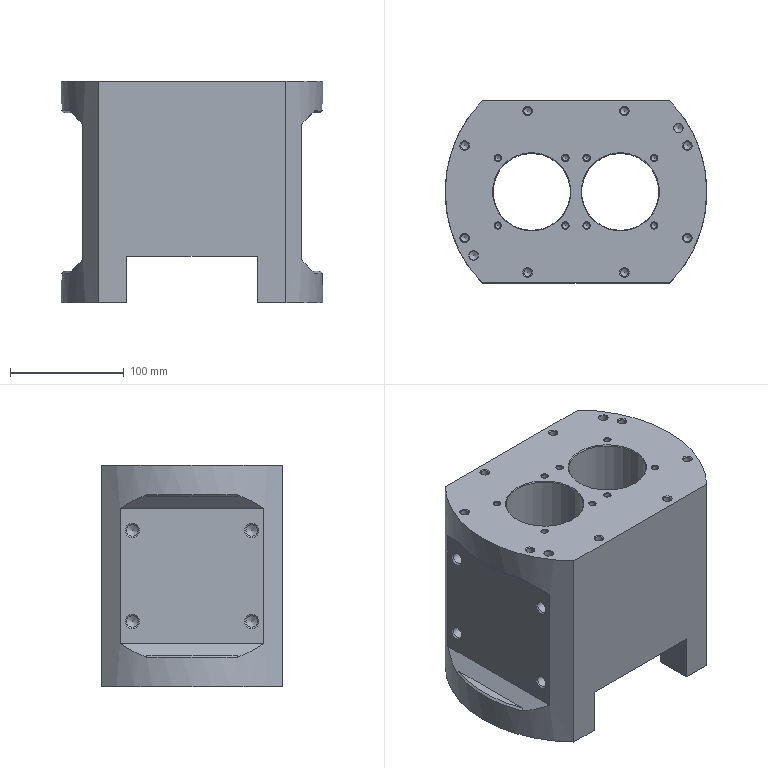NC program | NX | posted with a generic post | part box 230 x 160 x 195 mm
Whole program:
N10 G17 G21 G94 G90
(FLOOR_WALL , TOOL : D50)
N12 T02 M6
N14 G54
N16 G17 G0 G90 X-46.956 Y107.497 B0. C0. S1200 M3
N18 G43 Z30. H2
N20 Z2.651
N22 G94 G1 Z-0.349 F1000.
N24 X-43.956
N26 X43.956 F2000.
N28 Y68.498
N30 X-43.956
N32 Y29.498
N34 X43.956
N36 Y-9.501
N38 X-43.956
N40 Y-48.501
N42 X43.956
N44 Y-87.5
N46 X-43.956
N48 X-46.956
N50 Z2.651
N52 G0 Z30.
N54 X-50.654 Y107.497
N56 Z2.302
N58 G1 Z-0.698 F1000.
N60 X-47.654
N62 X47.654 F2000.
N64 Y68.498
N66 X-47.654
N68 Y29.498
N70 X47.654
N72 Y-9.501
N74 X-47.654
N76 Y-48.501
N78 X47.654
N80 Y-87.5
N82 X-47.654
N84 X-50.654
N86 Z2.302
N88 G0 Z30.
N90 X-53.485 Y107.497
N92 Z1.953
N94 G1 Z-1.047 F1000.
N96 X-50.485
N98 X50.485 F2000.
N100 Y68.498
N102 X-50.485
N104 Y29.498
N106 X50.485
N108 Y-9.501
N110 X-50.485
N112 Y-48.501
N114 X50.485
N116 Y-87.5
N118 X-50.485
N120 X-53.485
N122 Z1.953
N124 G0 Z30.
N126 X-55.866 Y107.497
N128 Z1.604
N130 G1 Z-1.396 F1000.
N132 X-52.866
N134 X52.866 F2000.
N136 Y68.498
N138 X-52.866
N140 Y29.498
N142 X52.866
N144 Y-9.501
N146 X-52.866
N148 Y-48.501
N150 X52.866
N152 Y-87.5
N154 X-52.866
N156 X-55.866
N158 Z1.604
N160 G0 Z30.
N162 X-57.959 Y107.497
N164 Z1.255
N166 G1 Z-1.745 F1000.
N168 X-54.959
N170 X54.959 F2000.
N172 Y68.498
N174 X-54.959
N176 Y29.498
N178 X54.959
N180 Y-9.501
N182 X-54.959
N184 Y-48.501
N186 X54.959
N188 Y-87.5
N190 X-54.959
N192 X-57.959
N194 Z1.255
N196 G0 Z30.
N198 X-59.847 Y107.497
N200 Z0.906
N202 G1 Z-2.094 F1000.
N204 X-56.847
N206 X56.847 F2000.
N208 Y68.498
N210 X-56.847
N212 Y29.498
N214 X56.847
N216 Y-9.501
N218 X-56.847
N220 Y-48.501
N222 X56.847
N224 Y-87.5
N226 X-56.847
N228 X-59.847
N230 Z0.906
N232 G0 Z30.
N234 X-61.579 Y107.497
N236 Z0.557
N238 G1 Z-2.443 F1000.
N240 X-58.579
N242 X58.579 F2000.
N244 Y68.498
N246 X-58.579
N248 Y29.498
N250 X58.579
N252 Y-9.501
N254 X-58.579
N256 Y-48.501
N258 X58.579
N260 Y-87.5
N262 X-58.579
N264 X-61.579
N266 Z0.557
N268 G0 Z30.
N270 X-63.188 Y107.497
N272 Z0.208
N274 G1 Z-2.792 F1000.
N276 X-60.188
N278 X60.188 F2000.
N280 Y68.498
N282 X-60.188
N284 Y29.498
N286 X60.188
N288 Y-9.501
N290 X-60.188
N292 Y-48.501
N294 X60.188
N296 Y-87.5
N298 X-60.188
N300 X-63.188
N302 Z0.208
N304 G0 Z30.
N306 X-64.695 Y107.497
N308 Z-0.141
N310 G1 Z-3.141 F1000.
N312 X-61.695
N314 X61.695 F2000.
N316 Y68.498
N318 X-61.695
N320 Y29.498
N322 X61.695
N324 Y-9.501
N326 X-61.695
N328 Y-48.501
N330 X61.695
N332 Y-87.5
N334 X-61.695
N336 X-64.695
N338 Z-0.141
N340 G0 Z30.
N342 X-66.117 Y107.497
N344 Z-0.49
N346 G1 Z-3.49 F1000.
N348 X-63.117
N350 X63.117 F2000.
N352 Y68.498
N354 X-63.117
N356 Y29.498
N358 X63.117
N360 Y-9.501
N362 X-63.117
N364 Y-48.501
N366 X63.117
N368 Y-87.5
N370 X-63.117
N372 X-66.117
N374 Z-0.49
N376 G0 Z30.
N378 X-67.467 Y107.497
N380 Z-0.839
N382 G1 Z-3.839 F1000.
N384 X-64.467
N386 X64.467 F2000.
N388 Y68.498
N390 X-64.467
N392 Y29.498
N394 X64.467
N396 Y-9.501
N398 X-64.467
N400 Y-48.501
N402 X64.467
N404 Y-87.5
N406 X-64.467
N408 X-67.467
N410 Z-0.839
N412 G0 Z30.
N414 X-68.753 Y107.497
N416 Z-1.188
N418 G1 Z-4.188 F1000.
N420 X-65.753
N422 X65.753 F2000.
N424 Y68.498
N426 X-65.753
N428 Y29.498
N430 X65.753
N432 Y-9.501
N434 X-65.753
N436 Y-48.501
N438 X65.753
N440 Y-87.5
N442 X-65.753
N444 X-68.753
N446 Z-1.188
N448 G0 Z30.
N450 X-69.984 Y107.497
N452 Z-1.537
N454 G1 Z-4.537 F1000.
N456 X-66.984
N458 X66.984 F2000.
N460 Y68.498
N462 X-66.984
N464 Y29.498
N466 X66.984
N468 Y-9.501
N470 X-66.984
N472 Y-48.501
N474 X66.984
N476 Y-87.5
N478 X-66.984
N480 X-69.984
N482 Z-1.537
N484 G0 Z30.
N486 X-71.166 Y107.497
N488 Z-1.886
N490 G1 Z-4.886 F1000.
N492 X-68.166
N494 X68.166 F2000.
N496 Y68.498
N498 X-68.166
N500 Y29.498
N502 X68.166
N504 Y-9.501
N506 X-68.166
N508 Y-48.501
N510 X68.166
N512 Y-87.5
N514 X-68.166
N516 X-71.166
N518 Z-1.886
N520 G0 Z30.
N522 X-72.303 Y107.497
N524 Z-2.235
N526 G1 Z-5.235 F1000.
N528 X-69.303
N530 X69.303 F2000.
N532 Y68.498
N534 X-69.303
N536 Y29.498
N538 X69.303
N540 Y-9.501
N542 X-69.303
N544 Y-48.501
N546 X69.303
N548 Y-87.5
N550 X-69.303
N552 X-72.303
N554 Z-2.235
N556 G0 Z30.
N558 X-73.4 Y107.497
N560 Z-2.584
N562 G1 Z-5.584 F1000.
N564 X-70.4
N566 X70.4 F2000.
N568 Y68.498
N570 X-70.4
N572 Y29.498
N574 X70.4
N576 Y-9.501
N578 X-70.4
N580 Y-48.501
N582 X70.4
N584 Y-87.5
N586 X-70.4
N588 X-73.4
N590 Z-2.584
N592 G0 Z30.
N594 X-74.462 Y107.497
N596 Z-2.933
N598 G1 Z-5.933 F1000.
N600 X-71.462
N602 X71.462 F2000.
N604 Y68.498
N606 X-71.462
N608 Y29.498
N610 X71.462
N612 Y-9.501
N614 X-71.462
N616 Y-48.501
N618 X71.462
N620 Y-87.5
N622 X-71.462
N624 X-74.462
N626 Z-2.933
N628 G0 Z30.
N630 X-75.489 Y107.497
N632 Z-3.282
N634 G1 Z-6.282 F1000.
N636 X-72.489
N638 X72.489 F2000.
N640 Y68.498
N642 X-72.489
N644 Y29.498
N646 X72.489
N648 Y-9.501
N650 X-72.489
N652 Y-48.501
N654 X72.489
N656 Y-87.5
N658 X-72.489
N660 X-75.489
N662 Z-3.282
N664 G0 Z30.
N666 X-76.487 Y107.497
N668 Z-3.631
N670 G1 Z-6.631 F1000.
N672 X-73.487
N674 X73.487 F2000.
N676 Y68.498
N678 X-73.487
N680 Y29.498
N682 X73.487
N684 Y-9.501
N686 X-73.487
N688 Y-48.501
N690 X73.487
N692 Y-87.5
N694 X-73.487
N696 X-76.487
N698 Z-3.631
N700 G0 Z30.
N702 X-77.455 Y107.497
N704 Z-3.98
N706 G1 Z-6.98 F1000.
N708 X-74.455
N710 X74.455 F2000.
N712 Y68.498
N714 X-74.455
N716 Y29.498
N718 X74.455
N720 Y-9.501
N722 X-74.455
N724 Y-48.501
N726 X74.455
N728 Y-87.5
N730 X-74.455
N732 X-77.455
N734 Z-3.98
N736 G0 Z30.
N738 X-78.398 Y107.497
N740 Z-4.329
N742 G1 Z-7.329 F1000.
N744 X-75.398
N746 X75.398 F2000.
N748 Y68.498
N750 X-75.398
N752 Y29.498
N754 X75.398
N756 Y-9.501
N758 X-75.398
N760 Y-48.501
N762 X75.398
N764 Y-87.5
N766 X-75.398
N768 X-78.398
N770 Z-4.329
N772 G0 Z30.
N774 X-79.316 Y107.497
N776 Z-4.678
N778 G1 Z-7.678 F1000.
N780 X-76.316
N782 X76.316 F2000.
N784 Y68.498
N786 X-76.316
N788 Y29.498
N790 X76.316
N792 Y-9.501
N794 X-76.316
N796 Y-48.501
N798 X76.316
N800 Y-87.5
N802 X-76.316
N804 X-79.316
N806 Z-4.678
N808 G0 Z30.
N810 X-80.212 Y107.497
N812 Z-5.027
N814 G1 Z-8.027 F1000.
N816 X-77.212
N818 X77.212 F2000.
N820 Y68.498
N822 X-77.212
N824 Y29.498
N826 X77.212
N828 Y-9.501
N830 X-77.212
N832 Y-48.501
N834 X77.212
N836 Y-87.5
N838 X-77.212
N840 X-80.212
N842 Z-5.027
N844 G0 Z30.
N846 X-81.086 Y107.497
N848 Z-5.376
N850 G1 Z-8.376 F1000.
N852 X-78.086
N854 X78.086 F2000.
N856 Y68.498
N858 X-78.086
N860 Y29.498
N862 X78.086
N864 Y-9.501
N866 X-78.086
N868 Y-48.501
N870 X78.086
N872 Y-87.5
N874 X-78.086
N876 X-81.086
N878 Z-5.376
N880 G0 Z30.
N882 X-81.939 Y107.497
N884 Z-5.725
N886 G1 Z-8.725 F1000.
N888 X-78.939
N890 X78.939 F2000.
N892 Y68.498
N894 X-78.939
N896 Y29.498
N898 X78.939
N900 Y-9.501
N902 X-78.939
N904 Y-48.501
N906 X78.939
N908 Y-87.5
N910 X-78.939
N912 X-81.939
N914 Z-5.725
N916 G0 Z30.
N918 X-82.774 Y107.497
N920 Z-6.074
N922 G1 Z-9.074 F1000.
N924 X-79.774
N926 X79.774 F2000.
N928 Y68.498
N930 X-79.774
N932 Y29.498
N934 X79.774
N936 Y-9.501
N938 X-79.774
N940 Y-48.501
N942 X79.774
N944 Y-87.5
N946 X-79.774
N948 X-82.774
N950 Z-6.074
N952 G0 Z30.
N954 X-83.591 Y107.497
N956 Z-6.423
N958 G1 Z-9.423 F1000.
N960 X-80.591
N962 X80.591 F2000.
N964 Y68.498
N966 X-80.591
N968 Y29.498
N970 X80.591
N972 Y-9.501
N974 X-80.591
N976 Y-48.501
N978 X80.591
N980 Y-87.5
N982 X-80.591
N984 X-83.591
N986 Z-6.423
N988 G0 Z30.
N990 X-84.391 Y107.497
N992 Z-6.772
N994 G1 Z-9.772 F1000.
N996 X-81.391
N998 X81.391 F2000.
N1000 Y68.498
N1002 X-81.391
N1004 Y29.498
N1006 X81.391
N1008 Y-9.501
N1010 X-81.391
N1012 Y-48.501
N1014 X81.391
N1016 Y-87.5
N1018 X-81.391
N1020 X-84.391
N1022 Z-6.772
N1024 G0 Z30.
N1026 X-85.175 Y107.497
N1028 Z-7.121
N1030 G1 Z-10.121 F1000.
N1032 X-82.175
N1034 X82.175 F2000.
N1036 Y68.498
N1038 X-82.175
N1040 Y29.498
N1042 X82.175
N1044 Y-9.501
N1046 X-82.175
N1048 Y-48.501
N1050 X82.175
N1052 Y-87.5
N1054 X-82.175
N1056 X-85.175
N1058 Z-7.121
N1060 G0 Z30.
N1062 X-85.943 Y107.497
N1064 Z-7.47
N1066 G1 Z-10.47 F1000.
N1068 X-82.943
N1070 X82.943 F2000.
N1072 Y68.498
N1074 X-82.943
N1076 Y29.498
N1078 X82.943
N1080 Y-9.501
N1082 X-82.943
N1084 Y-48.501
N1086 X82.943
N1088 Y-87.5
N1090 X-82.943
N1092 X-85.943
N1094 Z-7.47
N1096 G0 Z30.
N1098 X-86.697 Y107.497
N1100 Z-7.819
N1102 G1 Z-10.819 F1000.
N1104 X-83.697
N1106 X83.697 F2000.
N1108 Y68.498
N1110 X-83.697
N1112 Y29.498
N1114 X83.697
N1116 Y-9.501
N1118 X-83.697
N1120 Y-48.501
N1122 X83.697
N1124 Y-87.5
N1126 X-83.697
N1128 X-86.697
N1130 Z-7.819
N1132 G0 Z30.
N1134 X-87.436 Y107.497
N1136 Z-8.168
N1138 G1 Z-11.168 F1000.
N1140 X-84.436
N1142 X84.436 F2000.
N1144 Y68.498
N1146 X-84.436
N1148 Y29.498
N1150 X84.436
N1152 Y-9.501
N1154 X-84.436
N1156 Y-48.501
N1158 X84.436
N1160 Y-87.5
N1162 X-84.436
N1164 X-87.436
N1166 Z-8.168
N1168 G0 Z30.
N1170 X-88.163 Y107.497
N1172 Z-8.517
N1174 G1 Z-11.517 F1000.
N1176 X-85.163
N1178 X85.163 F2000.
N1180 Y68.498
N1182 X-85.163
N1184 Y29.498
N1186 X85.163
N1188 Y-9.501
N1190 X-85.163
N1192 Y-48.501
N1194 X85.163
N1196 Y-87.5
N1198 X-85.163
N1200 X-88.163
N1202 Z-8.517
N1204 G0 Z30.
N1206 X-88.877 Y107.497
N1208 Z-8.866
N1210 G1 Z-11.866 F1000.
N1212 X-85.877
N1214 X85.877 F2000.
N1216 Y68.498
N1218 X-85.877
N1220 Y29.498
N1222 X85.877
N1224 Y-9.501
N1226 X-85.877
N1228 Y-48.501
N1230 X85.877
N1232 Y-87.5
N1234 X-85.877
N1236 X-88.877
N1238 Z-8.866
N1240 G0 Z30.
N1242 X-89.578 Y107.497
N1244 Z-9.215
N1246 G1 Z-12.215 F1000.
N1248 X-86.578
N1250 X86.578 F2000.
N1252 Y68.498
N1254 X-86.578
N1256 Y29.498
N1258 X86.578
N1260 Y-9.501
N1262 X-86.578
N1264 Y-48.501
N1266 X86.578
N1268 Y-87.5
N1270 X-86.578
N1272 X-89.578
N1274 Z-9.215
N1276 G0 Z30.
N1278 X-90.268 Y107.497
N1280 Z-9.564
N1282 G1 Z-12.564 F1000.
N1284 X-87.268
N1286 X87.268 F2000.
N1288 Y68.498
N1290 X-87.268
N1292 Y29.498
N1294 X87.268
N1296 Y-9.501
N1298 X-87.268
N1300 Y-48.501
N1302 X87.268
N1304 Y-87.5
N1306 X-87.268
N1308 X-90.268
N1310 Z-9.564
N1312 G0 Z30.
N1314 X-90.946 Y107.497
N1316 Z-9.913
N1318 G1 Z-12.913 F1000.
N1320 X-87.946
N1322 X87.946 F2000.
N1324 Y68.498
N1326 X-87.946
N1328 Y29.498
N1330 X87.946
N1332 Y-9.501
N1334 X-87.946
N1336 Y-48.501
N1338 X87.946
N1340 Y-87.5
N1342 X-87.946
N1344 X-90.946
N1346 Z-9.913
N1348 G0 Z30.
N1350 X-91.614 Y107.497
N1352 Z-10.262
N1354 G1 Z-13.262 F1000.
N1356 X-88.614
N1358 X88.614 F2000.
N1360 Y68.498
N1362 X-88.614
N1364 Y29.498
N1366 X88.614
N1368 Y-9.501
N1370 X-88.614
N1372 Y-48.501
N1374 X88.614
N1376 Y-87.5
N1378 X-88.614
N1380 X-91.614
N1382 Z-10.262
N1384 G0 Z30.
N1386 X-92.271 Y107.497
N1388 Z-10.611
N1390 G1 Z-13.611 F1000.
N1392 X-89.271
N1394 X89.271 F2000.
N1396 Y68.498
N1398 X-89.271
N1400 Y29.498
N1402 X89.271
N1404 Y-9.501
N1406 X-89.271
N1408 Y-48.501
N1410 X89.271
N1412 Y-87.5
N1414 X-89.271
N1416 X-92.271
N1418 Z-10.611
N1420 G0 Z30.
N1422 X-92.918 Y107.497
N1424 Z-10.96
N1426 G1 Z-13.96 F1000.
N1428 X-89.918
N1430 X89.918 F2000.
N1432 Y68.498
N1434 X-89.918
N1436 Y29.498
N1438 X89.918
N1440 Y-9.501
N1442 X-89.918
N1444 Y-48.501
N1446 X89.918
N1448 Y-87.5
N1450 X-89.918
N1452 X-92.918
N1454 Z-10.96
N1456 G0 Z30.
N1458 X-93.555 Y107.497
N1460 Z-11.309
N1462 G1 Z-14.309 F1000.
N1464 X-90.555
N1466 X90.555 F2000.
N1468 Y68.498
N1470 X-90.555
N1472 Y29.498
N1474 X90.555
N1476 Y-9.501
N1478 X-90.555
N1480 Y-48.501
N1482 X90.555
N1484 Y-87.5
N1486 X-90.555
N1488 X-93.555
N1490 Z-11.309
N1492 G0 Z30.
N1494 X-94.183 Y107.497
N1496 Z-11.658
N1498 G1 Z-14.658 F1000.
N1500 X-91.183
N1502 X91.183 F2000.
N1504 Y68.498
N1506 X-91.183
N1508 Y29.498
N1510 X91.183
N1512 Y-9.501
N1514 X-91.183
N1516 Y-48.501
N1518 X91.183
N1520 Y-87.5
N1522 X-91.183
N1524 X-94.183
N1526 Z-11.658
N1528 G0 Z30.
N1530 X-94.802 Y107.497
N1532 Z-12.007
N1534 G1 Z-15.007 F1000.
N1536 X-91.802
N1538 X91.802 F2000.
N1540 Y68.498
N1542 X-91.802
N1544 Y29.498
N1546 X91.802
N1548 Y-9.501
N1550 X-91.802
N1552 Y-48.501
N1554 X91.802
N1556 Y-87.5
N1558 X-91.802
N1560 X-94.802
N1562 Z-12.007
N1564 G0 Z30.
N1566 X-95.412 Y107.497
N1568 Z-12.356
N1570 G1 Z-15.356 F1000.
N1572 X-92.412
N1574 X92.412 F2000.
N1576 Y68.498
N1578 X-92.412
N1580 Y29.498
N1582 X92.412
N1584 Y-9.501
N1586 X-92.412
N1588 Y-48.501
N1590 X92.412
N1592 Y-87.5
N1594 X-92.412
N1596 X-95.412
N1598 Z-12.356
N1600 G0 Z30.
N1602 X-96.013 Y107.497
N1604 Z-12.705
N1606 G1 Z-15.705 F1000.
N1608 X-93.013
N1610 X93.013 F2000.
N1612 Y68.498
N1614 X-93.013
N1616 Y29.498
N1618 X93.013
N1620 Y-9.501
N1622 X-93.013
N1624 Y-48.501
N1626 X93.013
N1628 Y-87.5
N1630 X-93.013
N1632 X-96.013
N1634 Z-12.705
N1636 G0 Z30.
N1638 X-96.606 Y107.497
N1640 Z-13.054
N1642 G1 Z-16.054 F1000.
N1644 X-93.606
N1646 X93.606 F2000.
N1648 Y68.498
N1650 X-93.606
N1652 Y29.498
N1654 X93.606
N1656 Y-9.501
N1658 X-93.606
N1660 Y-48.501
N1662 X93.606
N1664 Y-87.5
N1666 X-93.606
N1668 X-96.606
N1670 Z-13.054
N1672 G0 Z30.
N1674 X-97.192 Y107.497
N1676 Z-13.403
N1678 G1 Z-16.403 F1000.
N1680 X-94.192
N1682 X94.192 F2000.
N1684 Y68.498
N1686 X-94.192
N1688 Y29.498
N1690 X94.192
N1692 Y-9.501
N1694 X-94.192
N1696 Y-48.501
N1698 X94.192
N1700 Y-87.5
N1702 X-94.192
N1704 X-97.192
N1706 Z-13.403
N1708 G0 Z30.
N1710 X-97.769 Y107.497
N1712 Z-13.752
N1714 G1 Z-16.752 F1000.
N1716 X-94.769
N1718 X94.769 F2000.
N1720 Y68.498
N1722 X-94.769
N1724 Y29.498
N1726 X94.769
N1728 Y-9.501
N1730 X-94.769
N1732 Y-48.501
N1734 X94.769
N1736 Y-87.5
N1738 X-94.769
N1740 X-97.769
N1742 Z-13.752
N1744 G0 Z30.
N1746 X-98.339 Y107.497
N1748 Z-14.101
N1750 G1 Z-17.101 F1000.
N1752 X-95.339
N1754 X95.339 F2000.
N1756 Y68.498
N1758 X-95.339
N1760 Y29.498
N1762 X95.339
N1764 Y-9.501
N1766 X-95.339
N1768 Y-48.501
N1770 X95.339
N1772 Y-87.5
N1774 X-95.339
N1776 X-98.339
N1778 Z-14.101
N1780 G0 Z30.
N1782 X-98.902 Y107.497
N1784 Z-14.45
N1786 G1 Z-17.45 F1000.
N1788 X-95.902
N1790 X95.902 F2000.
N1792 Y68.498
N1794 X-95.902
N1796 Y29.498
N1798 X95.902
N1800 Y-9.501
N1802 X-95.902
N1804 Y-48.501
N1806 X95.902
N1808 Y-87.5
N1810 X-95.902
N1812 X-98.902
N1814 Z-14.45
N1816 G0 Z30.
N1818 X-99.457 Y107.497
N1820 Z-14.799
N1822 G1 Z-17.799 F1000.
N1824 X-96.457
N1826 X96.457 F2000.
N1828 Y68.498
N1830 X-96.457
N1832 Y29.498
N1834 X96.457
N1836 Y-9.501
N1838 X-96.457
N1840 Y-48.501
N1842 X96.457
N1844 Y-87.5
N1846 X-96.457
N1848 X-99.457
N1850 Z-14.799
N1852 G0 Z30.
N1854 X-100.006 Y107.497
N1856 Z-15.148
N1858 G1 Z-18.148 F1000.
N1860 X-97.006
N1862 X97.006 F2000.
N1864 Y68.498
N1866 X-97.006
N1868 Y29.498
N1870 X97.006
N1872 Y-9.501
N1874 X-97.006
N1876 Y-48.501
N1878 X97.006
N1880 Y-87.5
N1882 X-97.006
N1884 X-100.006
N1886 Z-15.148
N1888 G0 Z30.
N1890 X-100.548 Y107.497
N1892 Z-15.497
N1894 G1 Z-18.497 F1000.
N1896 X-97.548
N1898 X97.548 F2000.
N1900 Y68.498
N1902 X-97.548
N1904 Y29.498
N1906 X97.548
N1908 Y-9.501
N1910 X-97.548
N1912 Y-48.501
N1914 X97.548
N1916 Y-87.5
N1918 X-97.548
N1920 X-100.548
N1922 Z-15.497
N1924 G0 Z30.
N1926 X-101.083 Y107.497
N1928 Z-15.846
N1930 G1 Z-18.846 F1000.
N1932 X-98.083
N1934 X98.083 F2000.
N1936 Y68.498
N1938 X-98.083
N1940 Y29.498
N1942 X98.083
N1944 Y-9.501
N1946 X-98.083
N1948 Y-48.501
N1950 X98.083
N1952 Y-87.5
N1954 X-98.083
N1956 X-101.083
N1958 Z-15.846
N1960 G0 Z30.
N1962 X-101.612 Y107.497
N1964 Z-16.195
N1966 G1 Z-19.195 F1000.
N1968 X-98.612
N1970 X98.612 F2000.
N1972 Y68.498
N1974 X-98.612
N1976 Y29.498
N1978 X98.612
N1980 Y-9.501
N1982 X-98.612
N1984 Y-48.501
N1986 X98.612
N1988 Y-87.5
N1990 X-98.612
N1992 X-101.612
N1994 Z-16.195
N1996 G0 Z30.
N1998 X-102.134 Y107.497
N2000 Z-16.544
N2002 G1 Z-19.544 F1000.
N2004 X-99.134
N2006 X99.134 F2000.
N2008 Y68.498
N2010 X-99.134
N2012 Y29.498
N2014 X99.134
N2016 Y-9.501
N2018 X-99.134
N2020 Y-48.501
N2022 X99.134
N2024 Y-87.5
N2026 X-99.134
N2028 X-102.134
N2030 Z-16.544
N2032 G0 Z30.
N2034 X-102.65 Y107.497
N2036 Z-16.893
N2038 G1 Z-19.893 F1000.
N2040 X-99.65
N2042 X99.65 F2000.
N2044 Y68.498
N2046 X-99.65
N2048 Y29.498
N2050 X99.65
N2052 Y-9.501
N2054 X-99.65
N2056 Y-48.501
N2058 X99.65
N2060 Y-87.5
N2062 X-99.65
N2064 X-102.65
N2066 Z-16.893
N2068 G0 Z30.
N2070 X-103.161 Y107.497
N2072 Z-17.242
N2074 G1 Z-20.242 F1000.
N2076 X-100.161
N2078 X100.161 F2000.
N2080 Y68.498
N2082 X-100.161
N2084 Y29.498
N2086 X100.161
N2088 Y-9.501
N2090 X-100.161
N2092 Y-48.501
N2094 X100.161
N2096 Y-87.5
N2098 X-100.161
N2100 X-103.161
N2102 Z-17.242
N2104 G0 Z30.
N2106 X-103.666 Y107.497
N2108 Z-17.591
N2110 G1 Z-20.591 F1000.
N2112 X-100.666
N2114 X100.666 F2000.
N2116 Y68.498
N2118 X-100.666
N2120 Y29.498
N2122 X100.666
N2124 Y-9.501
N2126 X-100.666
N2128 Y-48.501
N2130 X100.666
N2132 Y-87.5
N2134 X-100.666
N2136 X-103.666
N2138 Z-17.591
N2140 G0 Z30.
N2142 X-104.164 Y107.497
N2144 Z-17.94
N2146 G1 Z-20.94 F1000.
N2148 X-101.164
N2150 X101.164 F2000.
N2152 Y68.498
N2154 X-101.164
N2156 Y29.498
N2158 X101.164
N2160 Y-9.501
N2162 X-101.164
N2164 Y-48.501
N2166 X101.164
N2168 Y-87.5
N2170 X-101.164
N2172 X-104.164
N2174 Z-17.94
N2176 G0 Z30.
N2178 X-104.658 Y107.497
N2180 Z-18.289
N2182 G1 Z-21.289 F1000.
N2184 X-101.658
N2186 X101.658 F2000.
N2188 Y68.498
N2190 X-101.658
N2192 Y29.498
N2194 X101.658
N2196 Y-9.501
N2198 X-101.658
N2200 Y-48.501
N2202 X101.658
N2204 Y-87.5
N2206 X-101.658
N2208 X-104.658
N2210 Z-18.289
N2212 G0 Z30.
N2214 X-105.146 Y107.497
N2216 Z-18.638
N2218 G1 Z-21.638 F1000.
N2220 X-102.146
N2222 X102.146 F2000.
N2224 Y68.498
N2226 X-102.146
N2228 Y29.498
N2230 X102.146
N2232 Y-9.501
N2234 X-102.146
N2236 Y-48.501
N2238 X102.146
N2240 Y-87.5
N2242 X-102.146
N2244 X-105.146
N2246 Z-18.638
N2248 G0 Z30.
N2250 X-105.628 Y107.497
N2252 Z-18.987
N2254 G1 Z-21.987 F1000.
N2256 X-102.628
N2258 X102.628 F2000.
N2260 Y68.498
N2262 X-102.628
N2264 Y29.498
N2266 X102.628
N2268 Y-9.501
N2270 X-102.628
N2272 Y-48.501
N2274 X102.628
N2276 Y-87.5
N2278 X-102.628
N2280 X-105.628
N2282 Z-18.987
N2284 G0 Z30.
N2286 X-106.106 Y107.497
N2288 Z-19.336
N2290 G1 Z-22.336 F1000.
N2292 X-103.106
N2294 X103.106 F2000.
N2296 Y68.498
N2298 X-103.106
N2300 Y29.498
N2302 X103.106
N2304 Y-9.501
N2306 X-103.106
N2308 Y-48.501
N2310 X103.106
N2312 Y-87.5
N2314 X-103.106
N2316 X-106.106
N2318 Z-19.336
N2320 G0 Z30.
N2322 X-106.578 Y107.497
N2324 Z-19.685
N2326 G1 Z-22.685 F1000.
N2328 X-103.578
N2330 X103.578 F2000.
N2332 Y68.498
N2334 X-103.578
N2336 Y29.498
N2338 X103.578
N2340 Y-9.501
N2342 X-103.578
N2344 Y-48.501
N2346 X103.578
N2348 Y-87.5
N2350 X-103.578
N2352 X-106.578
N2354 Z-19.685
N2356 G0 Z30.
N2358 X-107.045 Y107.497
N2360 Z-20.034
N2362 G1 Z-23.034 F1000.
N2364 X-104.045
N2366 X104.045 F2000.
N2368 Y68.498
N2370 X-104.045
N2372 Y29.498
N2374 X104.045
N2376 Y-9.501
N2378 X-104.045
N2380 Y-48.501
N2382 X104.045
N2384 Y-87.5
N2386 X-104.045
N2388 X-107.045
N2390 Z-20.034
N2392 G0 Z30.
N2394 X-107.508 Y107.497
N2396 Z-20.383
N2398 G1 Z-23.383 F1000.
N2400 X-104.508
N2402 X104.508 F2000.
N2404 Y68.498
N2406 X-104.508
N2408 Y29.498
N2410 X104.508
N2412 Y-9.501
N2414 X-104.508
N2416 Y-48.501
N2418 X104.508
N2420 Y-87.5
N2422 X-104.508
N2424 X-107.508
N2426 Z-20.383
N2428 G0 Z30.
N2430 X-107.965 Y107.497
N2432 Z-20.732
N2434 G1 Z-23.732 F1000.
N2436 X-104.965
N2438 X104.965 F2000.
N2440 Y68.498
N2442 X-104.965
N2444 Y29.498
N2446 X104.965
N2448 Y-9.501
N2450 X-104.965
N2452 Y-48.501
N2454 X104.965
N2456 Y-87.5
N2458 X-104.965
N2460 X-107.965
N2462 Z-20.732
N2464 G0 Z30.
N2466 X-108.418 Y107.497
N2468 Z-21.081
N2470 G1 Z-24.081 F1000.
N2472 X-105.418
N2474 X105.418 F2000.
N2476 Y68.498
N2478 X-105.418
N2480 Y29.498
N2482 X105.418
N2484 Y-9.501
N2486 X-105.418
N2488 Y-48.501
N2490 X105.418
N2492 Y-87.5
N2494 X-105.418
N2496 X-108.418
N2498 Z-21.081
N2500 G0 Z30.
N2502 X-108.867 Y107.497
N2504 Z-21.43
N2506 G1 Z-24.43 F1000.
N2508 X-105.867
N2510 X105.867 F2000.
N2512 Y68.498
N2514 X-105.867
N2516 Y29.498
N2518 X105.867
N2520 Y-9.501
N2522 X-105.867
N2524 Y-48.501
N2526 X105.867
N2528 Y-87.5
N2530 X-105.867
N2532 X-108.867
N2534 Z-21.43
N2536 G0 Z30.
N2538 X-109.31 Y107.497
N2540 Z-21.779
N2542 G1 Z-24.779 F1000.
N2544 X-106.31
N2546 X106.31 F2000.
N2548 Y68.498
N2550 X-106.31
N2552 Y29.498
N2554 X106.31
N2556 Y-9.501
N2558 X-106.31
N2560 Y-48.501
N2562 X106.31
N2564 Y-87.5
N2566 X-106.31
N2568 X-109.31
N2570 Z-21.779
N2572 G0 Z30.
N2574 X-109.75 Y107.497
N2576 Z-22.128
N2578 G1 Z-25.128 F1000.
N2580 X-106.75
N2582 X106.75 F2000.
N2584 Y68.498
N2586 X-106.75
N2588 Y29.498
N2590 X106.75
N2592 Y-9.501
N2594 X-106.75
N2596 Y-48.501
N2598 X106.75
N2600 Y-87.5
N2602 X-106.75
N2604 X-109.75
N2606 Z-22.128
N2608 G0 Z30.
N2610 X-110.185 Y107.497
N2612 Z-22.477
N2614 G1 Z-25.477 F1000.
N2616 X-107.185
N2618 X107.185 F2000.
N2620 Y68.498
N2622 X-107.185
N2624 Y29.498
N2626 X107.185
N2628 Y-9.501
N2630 X-107.185
N2632 Y-48.501
N2634 X107.185
N2636 Y-87.5
N2638 X-107.185
N2640 X-110.185
N2642 Z-22.477
N2644 G0 Z30.
N2646 X-110.616 Y107.497
N2648 Z-22.826
N2650 G1 Z-25.826 F1000.
N2652 X-107.616
N2654 X107.616 F2000.
N2656 Y68.498
N2658 X-107.616
N2660 Y29.498
N2662 X107.616
N2664 Y-9.501
N2666 X-107.616
N2668 Y-48.501
N2670 X107.616
N2672 Y-87.5
N2674 X-107.616
N2676 X-110.616
N2678 Z-22.826
N2680 G0 Z30.
N2682 X-111.042 Y107.497
N2684 Z-23.175
N2686 G1 Z-26.175 F1000.
N2688 X-108.042
N2690 X108.042 F2000.
N2692 Y68.498
N2694 X-108.042
N2696 Y29.498
N2698 X108.042
N2700 Y-9.501
N2702 X-108.042
N2704 Y-48.501
N2706 X108.042
N2708 Y-87.5
N2710 X-108.042
N2712 X-111.042
N2714 Z-23.175
N2716 G0 Z30.
N2718 X-111.464 Y107.497
N2720 Z-23.524
N2722 G1 Z-26.524 F1000.
N2724 X-108.464
N2726 X108.464 F2000.
N2728 Y68.498
N2730 X-108.464
N2732 Y29.498
N2734 X108.464
N2736 Y-9.501
N2738 X-108.464
N2740 Y-48.501
N2742 X108.464
N2744 Y-87.5
N2746 X-108.464
N2748 X-111.464
N2750 Z-23.524
N2752 G0 Z30.
N2754 X-111.883 Y107.497
N2756 Z-23.873
N2758 G1 Z-26.873 F1000.
N2760 X-108.883
N2762 X108.883 F2000.
N2764 Y68.498
N2766 X-108.883
N2768 Y29.498
N2770 X108.883
N2772 Y-9.501
N2774 X-108.883
N2776 Y-48.501
N2778 X108.883
N2780 Y-87.5
N2782 X-108.883
N2784 X-111.883
N2786 Z-23.873
N2788 G0 Z30.
N2790 X-112.297 Y107.497
N2792 Z-24.222
N2794 G1 Z-27.222 F1000.
N2796 X-109.297
N2798 X109.297 F2000.
N2800 Y68.498
N2802 X-109.297
N2804 Y29.498
N2806 X109.297
N2808 Y-9.501
N2810 X-109.297
N2812 Y-48.501
N2814 X109.297
N2816 Y-87.5
N2818 X-109.297
N2820 X-112.297
N2822 Z-24.222
N2824 G0 Z30.
N2826 X-112.707 Y107.497
N2828 Z-24.571
N2830 G1 Z-27.571 F1000.
N2832 X-109.707
N2834 X109.707 F2000.
N2836 Y68.498
N2838 X-109.707
N2840 Y29.498
N2842 X109.707
N2844 Y-9.501
N2846 X-109.707
N2848 Y-48.501
N2850 X109.707
N2852 Y-87.5
N2854 X-109.707
N2856 X-112.707
N2858 Z-24.571
N2860 G0 Z30.
N2862 X-113.114 Y107.497
N2864 Z-24.92
N2866 G1 Z-27.92 F1000.
N2868 X-110.114
N2870 X110.114 F2000.
N2872 Y68.498
N2874 X-110.114
N2876 Y29.498
N2878 X110.114
N2880 Y-9.501
N2882 X-110.114
N2884 Y-48.501
N2886 X110.114
N2888 Y-87.5
N2890 X-110.114
N2892 X-113.114
N2894 Z-24.92
N2896 G0 Z30.
N2898 X-113.517 Y107.497
N2900 Z-25.269
N2902 G1 Z-28.269 F1000.
N2904 X-110.517
N2906 X110.517 F2000.
N2908 Y68.498
N2910 X-110.517
N2912 Y29.498
N2914 X110.517
N2916 Y-9.501
N2918 X-110.517
N2920 Y-48.501
N2922 X110.517
N2924 Y-87.5
N2926 X-110.517
N2928 X-113.517
N2930 Z-25.269
N2932 G0 Z30.
N2934 X-113.915 Y107.497
N2936 Z-25.618
N2938 G1 Z-28.618 F1000.
N2940 X-110.915
N2942 X110.915 F2000.
N2944 Y68.498
N2946 X-110.915
N2948 Y29.498
N2950 X110.915
N2952 Y-9.501
N2954 X-110.915
N2956 Y-48.501
N2958 X110.915
N2960 Y-87.5
N2962 X-110.915
N2964 X-113.915
N2966 Z-25.618
N2968 G0 Z30.
N2970 X-114.311 Y107.497
N2972 Z-25.967
N2974 G1 Z-28.967 F1000.
N2976 X-111.311
N2978 X111.311 F2000.
N2980 Y68.498
N2982 X-111.311
N2984 Y29.498
N2986 X111.311
N2988 Y-9.501
N2990 X-111.311
N2992 Y-48.501
N2994 X111.311
N2996 Y-87.5
N2998 X-111.311
N3000 X-114.311
N3002 Z-25.967
N3004 G0 Z30.
N3006 X-114.702 Y107.497
N3008 Z-26.316
N3010 G1 Z-29.316 F1000.
N3012 X-111.702
N3014 X111.702 F2000.
N3016 Y68.498
N3018 X-111.702
N3020 Y29.498
N3022 X111.702
N3024 Y-9.501
N3026 X-111.702
N3028 Y-48.501
N3030 X111.702
N3032 Y-87.5
N3034 X-111.702
N3036 X-114.702
N3038 Z-26.316
N3040 G0 Z30.
N3042 X-115.091 Y107.497
N3044 Z-26.665
N3046 G1 Z-29.665 F1000.
N3048 X-112.091
N3050 X112.091 F2000.
N3052 Y68.498
N3054 X-112.091
N3056 Y29.498
N3058 X112.091
N3060 Y-9.501
N3062 X-112.091
N3064 Y-48.501
N3066 X112.091
N3068 Y-87.5
N3070 X-112.091
N3072 X-115.091
N3074 Z-26.665
N3076 G0 Z30.
N3078 X-115.475 Y107.497
N3080 Z-27.014
N3082 G1 Z-30.014 F1000.
N3084 X-112.475
N3086 X112.475 F2000.
N3088 Y68.498
N3090 X-112.475
N3092 Y29.498
N3094 X112.475
N3096 Y-9.501
N3098 X-112.475
N3100 Y-48.501
N3102 X112.475
N3104 Y-87.5
N3106 X-112.475
N3108 X-115.475
N3110 Z-27.014
N3112 G0 Z30.
N3114 X-115.856 Y107.497
N3116 Z-27.363
N3118 G1 Z-30.363 F1000.
N3120 X-112.856
N3122 X112.856 F2000.
N3124 Y68.498
N3126 X-112.856
N3128 Y29.498
N3130 X112.856
N3132 Y-9.501
N3134 X-112.856
N3136 Y-48.501
N3138 X112.856
N3140 Y-87.5
N3142 X-112.856
N3144 X-115.856
N3146 Z-27.363
N3148 G0 Z30.
N3150 X-116.234 Y107.497
N3152 Z-27.712
N3154 G1 Z-30.712 F1000.
N3156 X-113.234
N3158 X113.234 F2000.
N3160 Y68.498
N3162 X-113.234
N3164 Y29.498
N3166 X113.234
N3168 Y-9.501
N3170 X-113.234
N3172 Y-48.501
N3174 X113.234
N3176 Y-87.5
N3178 X-113.234
N3180 X-116.234
N3182 Z-27.712
N3184 G0 Z30.
N3186 X-116.608 Y107.497
N3188 Z-28.061
N3190 G1 Z-31.061 F1000.
N3192 X-113.608
N3194 X113.608 F2000.
N3196 Y68.498
N3198 X-113.608
N3200 Y29.498
N3202 X113.608
N3204 Y-9.501
N3206 X-113.608
N3208 Y-48.501
N3210 X113.608
N3212 Y-87.5
N3214 X-113.608
N3216 X-116.608
N3218 Z-28.061
N3220 G0 Z30.
N3222 X-116.979 Y107.497
N3224 Z-28.41
N3226 G1 Z-31.41 F1000.
N3228 X-113.979
N3230 X113.979 F2000.
N3232 Y68.498
N3234 X-113.979
N3236 Y29.498
N3238 X113.979
N3240 Y-9.501
N3242 X-113.979
N3244 Y-48.501
N3246 X113.979
N3248 Y-87.5
N3250 X-113.979
N3252 X-116.979
N3254 Z-28.41
N3256 G0 Z30.
N3258 X-117.347 Y107.497
N3260 Z-28.759
N3262 G1 Z-31.759 F1000.
N3264 X-114.347
N3266 X114.347 F2000.
N3268 Y68.498
N3270 X-114.347
N3272 Y29.498
N3274 X114.347
N3276 Y-9.501
N3278 X-114.347
N3280 Y-48.501
N3282 X114.347
N3284 Y-87.5
N3286 X-114.347
N3288 X-117.347
N3290 Z-28.759
N3292 G0 Z30.
N3294 X-117.711 Y107.497
N3296 Z-29.108
N3298 G1 Z-32.108 F1000.
N3300 X-114.711
N3302 X114.711 F2000.
N3304 Y68.498
N3306 X-114.711
N3308 Y29.498
N3310 X114.711
N3312 Y-9.501
N3314 X-114.711
N3316 Y-48.501
N3318 X114.711
N3320 Y-87.5
N3322 X-114.711
N3324 X-117.711
N3326 Z-29.108
N3328 G0 Z30.
N3330 X-118.073 Y107.497
N3332 Z-29.457
N3334 G1 Z-32.457 F1000.
N3336 X-115.073
N3338 X115.073 F2000.
N3340 Y68.498
N3342 X-115.073
N3344 Y29.498
N3346 X115.073
N3348 Y-9.501
N3350 X-115.073
N3352 Y-48.501
N3354 X115.073
N3356 Y-87.5
N3358 X-115.073
N3360 X-118.073
N3362 Z-29.457
N3364 G0 Z30.
N3366 X-118.431 Y107.497
N3368 Z-29.806
N3370 G1 Z-32.806 F1000.
N3372 X-115.431
N3374 X115.431 F2000.
N3376 Y68.498
N3378 X-115.431
N3380 Y29.498
N3382 X115.431
N3384 Y-9.501
N3386 X-115.431
N3388 Y-48.501
N3390 X115.431
N3392 Y-87.5
N3394 X-115.431
N3396 X-118.431
N3398 Z-29.806
N3400 G0 Z30.
N3402 X-118.786 Y107.497
N3404 Z-30.155
N3406 G1 Z-33.155 F1000.
N3408 X-115.786
N3410 X115.786 F2000.
N3412 Y68.498
N3414 X-115.786
N3416 Y29.498
N3418 X115.786
N3420 Y-9.501
N3422 X-115.786
N3424 Y-48.501
N3426 X115.786
N3428 Y-87.5
N3430 X-115.786
N3432 X-118.786
N3434 Z-30.155
N3436 G0 Z30.
N3438 X-119.138 Y107.497
N3440 Z-30.504
N3442 G1 Z-33.504 F1000.
N3444 X-116.138
N3446 X116.138 F2000.
N3448 Y68.498
N3450 X-116.138
N3452 Y29.498
N3454 X116.138
N3456 Y-9.501
N3458 X-116.138
N3460 Y-48.501
N3462 X116.138
N3464 Y-87.5
N3466 X-116.138
N3468 X-119.138
N3470 Z-30.504
N3472 G0 Z30.
N3474 X-119.487 Y107.497
N3476 Z-30.853
N3478 G1 Z-33.853 F1000.
N3480 X-116.487
N3482 X116.487 F2000.
N3484 Y68.498
N3486 X-116.487
N3488 Y29.498
N3490 X116.487
N3492 Y-9.501
N3494 X-116.487
N3496 Y-48.501
N3498 X116.487
N3500 Y-87.5
N3502 X-116.487
N3504 X-119.487
N3506 Z-30.853
N3508 G0 Z30.
N3510 X-119.833 Y107.497
N3512 Z-31.202
N3514 G1 Z-34.202 F1000.
N3516 X-116.833
N3518 X116.833 F2000.
N3520 Y68.498
N3522 X-116.833
N3524 Y29.498
N3526 X116.833
N3528 Y-9.501
N3530 X-116.833
N3532 Y-48.501
N3534 X116.833
N3536 Y-87.5
N3538 X-116.833
N3540 X-119.833
N3542 Z-31.202
N3544 G0 Z30.
N3546 X-120.176 Y107.497
N3548 Z-31.551
N3550 G1 Z-34.551 F1000.
N3552 X-117.176
N3554 X117.176 F2000.
N3556 Y68.498
N3558 X-117.176
N3560 Y29.498
N3562 X117.176
N3564 Y-9.501
N3566 X-117.176
N3568 Y-48.501
N3570 X117.176
N3572 Y-87.5
N3574 X-117.176
N3576 X-120.176
N3578 Z-31.551
N3580 G0 Z30.
N3582 X-120.517 Y107.497
N3584 Z-31.9
N3586 G1 Z-34.9 F1000.
N3588 X-117.517
N3590 X117.517 F2000.
N3592 Y68.498
N3594 X-117.517
N3596 Y29.498
N3598 X117.517
N3600 Y-9.501
N3602 X-117.517
N3604 Y-48.501
N3606 X117.517
N3608 Y-87.5
N3610 X-117.517
N3612 X-120.517
N3614 Z-31.9
N3616 G0 Z30.
(FLOOR_WALL_COPY , TOOL : D50)
N3618 X-120.614 Y107.497 S2500
N3620 Z-32.
N3622 G1 Z-35. F1000.
N3624 X-117.614
N3626 X117.614
N3628 Y68.498
N3630 X-117.614
N3632 Y29.498
N3634 X117.614
N3636 Y-9.501
N3638 X-117.614
N3640 Y-48.501
N3642 X117.614
N3644 Y-87.5
N3646 X-117.614
N3648 X-120.614
N3650 Z-32.
N3652 G0 Z30.
N3654 M5
(DRILLING , TOOL : ZXZ)
N3656 T01 M6
N3658 G54
N3660 G17 G0 G90 X52.5 Y17.5 B0. C0. S5000 M3
N3662 G43 Z30. H1
N3664 G94 G81 G98 Z-36. F250. R-32.
N3666 Y-62.5
N3668 X-52.5
N3670 Y17.5
N3672 G80
N3674 G0 X-52.5 Y17.5 Z30.
N3676 M5
(DRILLING_COPY , TOOL : 10.2ZT)
N3678 T11 M6
N3680 G54
N3682 G17 G0 G90 X52.5 Y17.5 B0. C0. S1200 M3
N3684 G43 Z30. H11
N3686 G94 G83 G98 Z-64.064 F250. Q2. R-32.
N3688 Y-62.5
N3690 X-52.5
N3692 Y17.5
N3694 G80
N3696 G0 X-52.5 Y17.5 Z30.
N3698 M5
(PLANAR_MILL_COPY_COPY , TOOL : D6A45)
N3700 T07 M6
N3702 G54
N3704 G17 G0 G90 X55.447 Y15.521 B0. C0. S7500 M3
N3706 G43 Z30. H7
N3708 Z-33.5
N3710 G94 G1 Z-36.5 F1250.
N3712 X56.893 Y16.734
N3714 G3 X57.25 Y17.5 R1.
N3716 X52.5 Y22.25 R4.75
N3718 X57.25 Y17.5 R-4.75
N3720 X56.893 Y18.266 R1.
N3722 G1 X55.447 Y19.479
N3724 Z-33.5
N3726 G0 Z30.
N3728 Y-64.479
N3730 Z-33.5
N3732 G1 Z-36.5
N3734 X56.893 Y-63.266
N3736 G3 X57.25 Y-62.5 R1.
N3738 X52.5 Y-57.75 R4.75
N3740 X57.25 Y-62.5 R-4.75
N3742 X56.893 Y-61.734 R1.
N3744 G1 X55.447 Y-60.521
N3746 Z-33.5
N3748 G0 Z30.
N3750 X-55.447
N3752 Z-33.5
N3754 G1 Z-36.5
N3756 X-56.893 Y-61.734
N3758 G3 X-57.25 Y-62.5 R1.
N3760 X-52.5 Y-67.25 R4.75
N3762 X-57.25 Y-62.5 R-4.75
N3764 X-56.893 Y-63.266 R1.
N3766 G1 X-55.447 Y-64.479
N3768 Z-33.5
N3770 G0 Z30.
N3772 Y19.479
N3774 Z-33.5
N3776 G1 Z-36.5
N3778 X-56.893 Y18.266
N3780 G3 X-57.25 Y17.5 R1.
N3782 X-52.5 Y12.75 R4.75
N3784 X-57.25 Y17.5 R-4.75
N3786 X-56.893 Y16.734 R1.
N3788 G1 X-55.447 Y15.521
N3790 Z-33.5
N3792 G0 Z30.
N3794 M5
N3796 M2